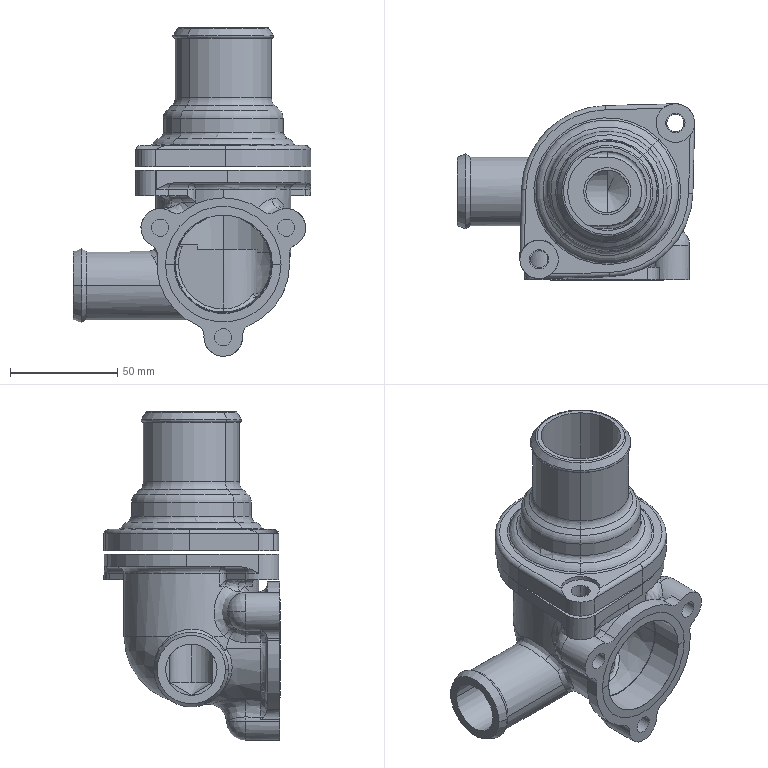Part | SolidWorks | features BaseBody 2 | 2 solids | 238 faces | box 110.82 x 82.273 x 153.5 mm | volume 186493 mm3 | cylinder 87 | torus 49 | plane 41 | spline 25 | cone 22 | sphere 14 | commonest cylinder face diameters 18 x15 8 x10 6 x9 10 x8 4 x4 9 x4